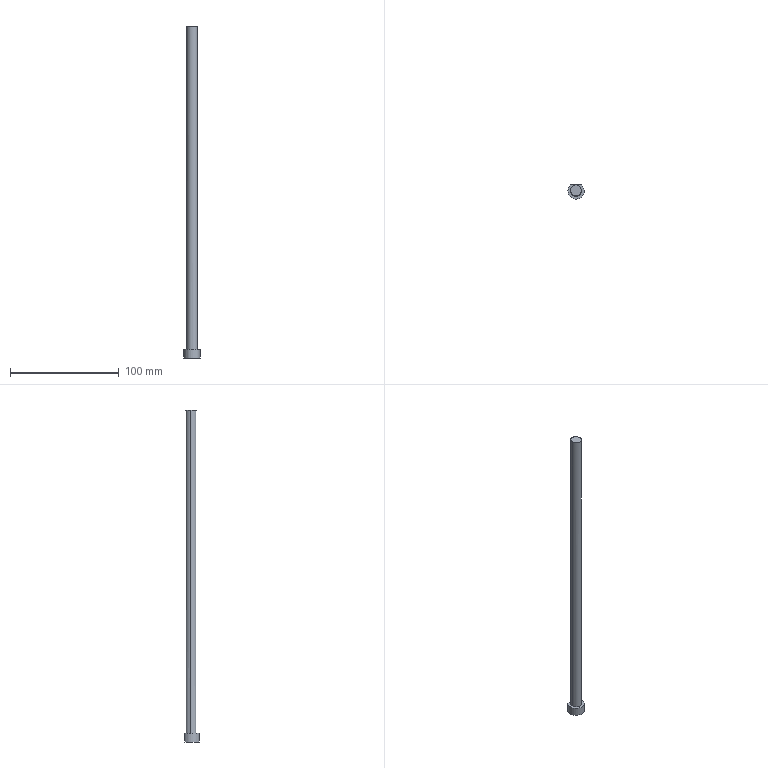Part | Creo | 1 solid | 7 faces | box 15 x 13 x 305.605 mm | volume 24670 mm3 | plane 4 | cylinder 3 | commonest cylinder face diameters 10 x2 15 x1
STEP:
#1=CARTESIAN_POINT('',(0.,0.,0.));
#2=DIRECTION('',(0.,0.,1.));
#3=DIRECTION('',(1.,0.,0.));
#4=AXIS2_PLACEMENT_3D('',#1,#2,#3);
#5=CARTESIAN_POINT('',(91.17,-165.946,-330.441));
#6=VERTEX_POINT('',#5);
#7=CARTESIAN_POINT('',(88.769,-171.446,-330.441));
#8=VERTEX_POINT('',#7);
#9=CARTESIAN_POINT('',(96.269,-171.446,-330.441));
#10=DIRECTION('',(0.,0.,1.));
#11=DIRECTION('',(-0.6799,0.7333,0.));
#12=AXIS2_PLACEMENT_3D('',#9,#10,#11);
#13=CIRCLE('',#12,7.5);
#14=EDGE_CURVE('',#6,#8,#13,.T.);
#15=ORIENTED_EDGE('',*,*,#14,.F.);
#16=CARTESIAN_POINT('',(101.368,-165.946,-330.441));
#17=VERTEX_POINT('',#16);
#18=CARTESIAN_POINT('',(91.17,-165.946,-330.441));
#19=DIRECTION('',(1.,0.,0.));
#20=VECTOR('',#19,10.198);
#21=LINE('',#18,#20);
#22=EDGE_CURVE('',#6,#17,#21,.T.);
#23=ORIENTED_EDGE('',*,*,#22,.T.);
#24=CARTESIAN_POINT('',(96.269,-171.446,-330.441));
#25=DIRECTION('',(0.,0.,1.));
#26=DIRECTION('',(-1.,0.,0.));
#27=AXIS2_PLACEMENT_3D('',#24,#25,#26);
#28=CIRCLE('',#27,7.5);
#29=EDGE_CURVE('',#8,#17,#28,.T.);
#30=ORIENTED_EDGE('',*,*,#29,.F.);
#31=EDGE_LOOP('',(#15,#23,#30));
#32=FACE_OUTER_BOUND('',#31,.F.);
#33=CARTESIAN_POINT('',(101.269,-171.446,-330.441));
#34=VERTEX_POINT('',#33);
#35=CARTESIAN_POINT('',(91.269,-171.446,-330.441));
#36=VERTEX_POINT('',#35);
#37=CARTESIAN_POINT('',(96.269,-171.446,-330.441));
#38=DIRECTION('',(0.,0.,-1.));
#39=DIRECTION('',(1.,0.,0.));
#40=AXIS2_PLACEMENT_3D('',#37,#38,#39);
#41=CIRCLE('',#40,5.);
#42=EDGE_CURVE('',#34,#36,#41,.T.);
#43=ORIENTED_EDGE('',*,*,#42,.F.);
#44=CARTESIAN_POINT('',(96.269,-171.446,-330.441));
#45=DIRECTION('',(0.,0.,-1.));
#46=DIRECTION('',(-1.,0.,0.));
#47=AXIS2_PLACEMENT_3D('',#44,#45,#46);
#48=CIRCLE('',#47,5.);
#49=EDGE_CURVE('',#36,#34,#48,.T.);
#50=ORIENTED_EDGE('',*,*,#49,.F.);
#51=EDGE_LOOP('',(#43,#50));
#52=FACE_BOUND('',#51,.F.);
#53=CARTESIAN_POINT('',(96.269,-171.446,-330.441));
#54=DIRECTION('',(0.,0.,1.));
#55=DIRECTION('',(1.,0.,0.));
#56=AXIS2_PLACEMENT_3D('',#53,#54,#55);
#57=PLANE('',#56);
#58=ADVANCED_FACE('',(#32,#52),#57,.T.);
#59=ORIENTED_EDGE('',*,*,#42,.T.);
#60=CARTESIAN_POINT('',(91.269,-171.446,-32.891));
#61=VERTEX_POINT('',#60);
#62=CARTESIAN_POINT('',(91.269,-171.446,-330.441));
#63=DIRECTION('',(0.,0.,1.));
#64=VECTOR('',#63,297.551);
#65=LINE('',#62,#64);
#66=EDGE_CURVE('',#36,#61,#65,.T.);
#67=ORIENTED_EDGE('',*,*,#66,.T.);
#68=CARTESIAN_POINT('',(101.269,-171.446,-32.972));
#69=VERTEX_POINT('',#68);
#70=CARTESIAN_POINT('',(91.269,-171.446,-32.891));
#71=CARTESIAN_POINT('',(91.269,-172.035,-32.901));
#72=CARTESIAN_POINT('',(91.484,-173.308,-32.925));
#73=CARTESIAN_POINT('',(92.625,-175.087,-32.965));
#74=CARTESIAN_POINT('',(94.42,-176.232,-32.999));
#75=CARTESIAN_POINT('',(96.269,-176.553,-33.02));
#76=CARTESIAN_POINT('',(98.119,-176.232,-33.029));
#77=CARTESIAN_POINT('',(99.914,-175.087,-33.024));
#78=CARTESIAN_POINT('',(101.055,-173.308,-33.003));
#79=CARTESIAN_POINT('',(101.269,-172.035,-32.982));
#80=CARTESIAN_POINT('',(101.269,-171.446,-32.972));
#81=B_SPLINE_CURVE_WITH_KNOTS('',3,(#70,#71,#72,#73,#74,#75,#76,#77,#78,#79,#80),.UNSPECIFIED.,.F.,.F.,(4,1,1,1,1,1,1,1,4),(0.,0.125,0.25,0.375,0.5,0.625,0.75,0.875,1.),.UNSPECIFIED.);
#82=EDGE_CURVE('',#61,#69,#81,.T.);
#83=ORIENTED_EDGE('',*,*,#82,.T.);
#84=CARTESIAN_POINT('',(101.269,-171.446,-330.441));
#85=DIRECTION('',(0.,0.,1.));
#86=VECTOR('',#85,297.469);
#87=LINE('',#84,#86);
#88=EDGE_CURVE('',#34,#69,#87,.T.);
#89=ORIENTED_EDGE('',*,*,#88,.F.);
#90=EDGE_LOOP('',(#59,#67,#83,#89));
#91=FACE_OUTER_BOUND('',#90,.F.);
#92=CARTESIAN_POINT('',(96.269,-171.446,-653.441));
#93=DIRECTION('',(0.,0.,1.));
#94=DIRECTION('',(1.,0.,0.));
#95=AXIS2_PLACEMENT_3D('',#92,#93,#94);
#96=CYLINDRICAL_SURFACE('',#95,5.);
#97=ADVANCED_FACE('',(#91),#96,.T.);
#98=ORIENTED_EDGE('',*,*,#49,.T.);
#99=ORIENTED_EDGE('',*,*,#88,.T.);
#100=CARTESIAN_POINT('',(94.14,-166.922,-32.836));
#101=VERTEX_POINT('',#100);
#102=CARTESIAN_POINT('',(101.269,-171.446,-32.972));
#103=CARTESIAN_POINT('',(101.269,-170.789,-32.961));
#104=CARTESIAN_POINT('',(101.053,-169.816,-32.942));
#105=CARTESIAN_POINT('',(100.324,-168.34,-32.911));
#106=CARTESIAN_POINT('',(99.022,-167.109,-32.879));
#107=CARTESIAN_POINT('',(97.353,-166.455,-32.854));
#108=CARTESIAN_POINT('',(95.706,-166.423,-32.84));
#109=CARTESIAN_POINT('',(94.734,-166.642,-32.836));
#110=B_SPLINE_CURVE_WITH_KNOTS('',3,(#102,#103,#104,#105,#106,#107,#108,#109,#100),.UNSPECIFIED.,.F.,.F.,(4,1,1,1,1,1,4),(0.,0.125,0.25,0.5,0.75,0.875,1.),.UNSPECIFIED.);
#111=EDGE_CURVE('',#69,#101,#110,.T.);
#112=ORIENTED_EDGE('',*,*,#111,.T.);
#113=CARTESIAN_POINT('',(94.14,-166.922,-32.836));
#114=CARTESIAN_POINT('',(93.183,-167.373,-32.836));
#115=CARTESIAN_POINT('',(91.869,-168.654,-32.848));
#116=CARTESIAN_POINT('',(91.269,-170.388,-32.873));
#117=CARTESIAN_POINT('',(91.269,-171.446,-32.891));
#118=B_SPLINE_CURVE_WITH_KNOTS('',3,(#113,#114,#115,#116,#117),.UNSPECIFIED.,.F.,.F.,(4,1,4),(0.,0.5,1.),.UNSPECIFIED.);
#119=EDGE_CURVE('',#101,#61,#118,.T.);
#120=ORIENTED_EDGE('',*,*,#119,.T.);
#121=ORIENTED_EDGE('',*,*,#66,.F.);
#122=EDGE_LOOP('',(#98,#99,#112,#120,#121));
#123=FACE_OUTER_BOUND('',#122,.F.);
#124=CARTESIAN_POINT('',(96.269,-171.446,-653.441));
#125=DIRECTION('',(0.,0.,1.));
#126=DIRECTION('',(1.,0.,0.));
#127=AXIS2_PLACEMENT_3D('',#124,#125,#126);
#128=CYLINDRICAL_SURFACE('',#127,5.);
#129=ADVANCED_FACE('',(#123),#128,.T.);
#130=ORIENTED_EDGE('',*,*,#119,.F.);
#131=ORIENTED_EDGE('',*,*,#111,.F.);
#132=ORIENTED_EDGE('',*,*,#82,.F.);
#133=EDGE_LOOP('',(#130,#131,#132));
#134=FACE_OUTER_BOUND('',#133,.F.);
#135=CARTESIAN_POINT('',(65.56,-187.537,-32.96));
#136=DIRECTION('',(-0.008129,0.01727,-0.9998));
#137=DIRECTION('',(0.,0.9999,0.01727));
#138=AXIS2_PLACEMENT_3D('',#135,#136,#137);
#139=PLANE('',#138);
#140=ADVANCED_FACE('',(#134),#139,.F.);
#141=CARTESIAN_POINT('',(101.368,-165.946,-338.441));
#142=VERTEX_POINT('',#141);
#143=CARTESIAN_POINT('',(101.368,-165.946,-338.441));
#144=DIRECTION('',(0.,0.,1.));
#145=VECTOR('',#144,8.);
#146=LINE('',#143,#145);
#147=EDGE_CURVE('',#142,#17,#146,.T.);
#148=ORIENTED_EDGE('',*,*,#147,.F.);
#149=CARTESIAN_POINT('',(88.769,-171.446,-338.441));
#150=VERTEX_POINT('',#149);
#151=CARTESIAN_POINT('',(96.269,-171.446,-338.441));
#152=DIRECTION('',(0.,0.,-1.));
#153=DIRECTION('',(0.6799,0.7333,0.));
#154=AXIS2_PLACEMENT_3D('',#151,#152,#153);
#155=CIRCLE('',#154,7.5);
#156=EDGE_CURVE('',#142,#150,#155,.T.);
#157=ORIENTED_EDGE('',*,*,#156,.T.);
#158=CARTESIAN_POINT('',(91.17,-165.946,-338.441));
#159=VERTEX_POINT('',#158);
#160=CARTESIAN_POINT('',(96.269,-171.446,-338.441));
#161=DIRECTION('',(0.,0.,-1.));
#162=DIRECTION('',(-1.,0.,0.));
#163=AXIS2_PLACEMENT_3D('',#160,#161,#162);
#164=CIRCLE('',#163,7.5);
#165=EDGE_CURVE('',#150,#159,#164,.T.);
#166=ORIENTED_EDGE('',*,*,#165,.T.);
#167=CARTESIAN_POINT('',(91.17,-165.946,-330.441));
#168=DIRECTION('',(0.,0.,-1.));
#169=VECTOR('',#168,8.);
#170=LINE('',#167,#169);
#171=EDGE_CURVE('',#6,#159,#170,.T.);
#172=ORIENTED_EDGE('',*,*,#171,.F.);
#173=ORIENTED_EDGE('',*,*,#14,.T.);
#174=ORIENTED_EDGE('',*,*,#29,.T.);
#175=EDGE_LOOP('',(#148,#157,#166,#172,#173,#174));
#176=FACE_OUTER_BOUND('',#175,.F.);
#177=CARTESIAN_POINT('',(96.269,-171.446,-330.441));
#178=DIRECTION('',(0.,0.,-1.));
#179=DIRECTION('',(-1.,0.,0.));
#180=AXIS2_PLACEMENT_3D('',#177,#178,#179);
#181=CYLINDRICAL_SURFACE('',#180,7.5);
#182=ADVANCED_FACE('',(#176),#181,.T.);
#183=ORIENTED_EDGE('',*,*,#22,.F.);
#184=ORIENTED_EDGE('',*,*,#171,.T.);
#185=CARTESIAN_POINT('',(101.368,-165.946,-338.441));
#186=DIRECTION('',(-1.,0.,0.));
#187=VECTOR('',#186,10.198);
#188=LINE('',#185,#187);
#189=EDGE_CURVE('',#142,#159,#188,.T.);
#190=ORIENTED_EDGE('',*,*,#189,.F.);
#191=ORIENTED_EDGE('',*,*,#147,.T.);
#192=EDGE_LOOP('',(#183,#184,#190,#191));
#193=FACE_OUTER_BOUND('',#192,.F.);
#194=CARTESIAN_POINT('',(96.269,-165.946,-338.441));
#195=DIRECTION('',(0.,1.,0.));
#196=DIRECTION('',(0.,0.,1.));
#197=AXIS2_PLACEMENT_3D('',#194,#195,#196);
#198=PLANE('',#197);
#199=ADVANCED_FACE('',(#193),#198,.T.);
#200=ORIENTED_EDGE('',*,*,#156,.F.);
#201=ORIENTED_EDGE('',*,*,#189,.T.);
#202=ORIENTED_EDGE('',*,*,#165,.F.);
#203=EDGE_LOOP('',(#200,#201,#202));
#204=FACE_OUTER_BOUND('',#203,.F.);
#205=CARTESIAN_POINT('',(71.601,-77.127,-338.441));
#206=DIRECTION('',(0.,0.,-1.));
#207=DIRECTION('',(-1.,0.,0.));
#208=AXIS2_PLACEMENT_3D('',#205,#206,#207);
#209=PLANE('',#208);
#210=ADVANCED_FACE('',(#204),#209,.T.);
#211=CLOSED_SHELL('',(#58,#97,#129,#140,#182,#199,#210));
#212=MANIFOLD_SOLID_BREP('',#211);
#213=(LENGTH_UNIT()NAMED_UNIT(*)SI_UNIT(.MILLI.,.METRE.));
#214=UNCERTAINTY_MEASURE_WITH_UNIT(LENGTH_MEASURE(0.03063),#213,'','');
#215=(NAMED_UNIT(*)PLANE_ANGLE_UNIT()SI_UNIT($,.RADIAN.));
#216=PLANE_ANGLE_MEASURE_WITH_UNIT(PLANE_ANGLE_MEASURE(0.01745),#215);
#217=(CONVERSION_BASED_UNIT('DEGREE',#216)NAMED_UNIT(*)PLANE_ANGLE_UNIT());
#218=(NAMED_UNIT(*)SI_UNIT($,.STERADIAN.)SOLID_ANGLE_UNIT());
#219=(GEOMETRIC_REPRESENTATION_CONTEXT(3)GLOBAL_UNCERTAINTY_ASSIGNED_CONTEXT((#214))GLOBAL_UNIT_ASSIGNED_CONTEXT((#213,#217,#218))REPRESENTATION_CONTEXT('',''));
#220=ADVANCED_BREP_SHAPE_REPRESENTATION('',(#4,#212),#219);